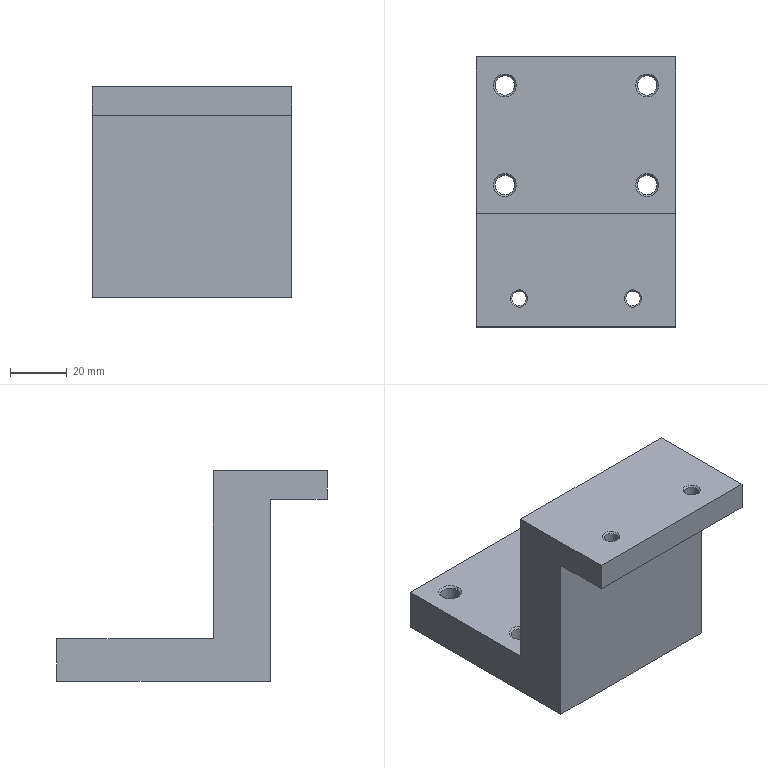Part | SolidWorks | features HoleWzd 2, ICE 2, Extrusion 1 | 1 solid | 34 faces | box 70 x 95 x 74 mm | volume 172756 mm3 | cone 12 | cylinder 12 | plane 10 | commonest cylinder face diameters 6.8 x8 5 x4
STEP:
#1=CARTESIAN_POINT('',(17.5,25.,9.475));
#2=VERTEX_POINT('',#1);
#3=CARTESIAN_POINT('',(22.5,25.,9.475));
#4=VERTEX_POINT('',#3);
#5=CARTESIAN_POINT('',(20.,25.,9.475));
#6=DIRECTION('',(0.,0.,1.));
#7=DIRECTION('',(1.,0.,0.));
#8=AXIS2_PLACEMENT_3D('',#5,#6,#7);
#9=CIRCLE('',#8,2.5);
#10=EDGE_CURVE('',#2,#4,#9,.T.);
#11=ORIENTED_EDGE('',*,*,#10,.F.);
#12=CARTESIAN_POINT('',(16.975,25.,10.));
#13=VERTEX_POINT('',#12);
#14=CARTESIAN_POINT('',(16.975,25.,10.));
#15=DIRECTION('',(-0.7071,0.,0.7071));
#16=VECTOR('',#15,1000.);
#17=LINE('',#14,#16);
#18=EDGE_CURVE('',#2,#13,#17,.T.);
#19=ORIENTED_EDGE('',*,*,#18,.T.);
#20=CARTESIAN_POINT('',(23.025,25.,10.));
#21=VERTEX_POINT('',#20);
#22=CARTESIAN_POINT('',(20.,25.,10.));
#23=DIRECTION('',(0.,0.,1.));
#24=DIRECTION('',(1.,0.,0.));
#25=AXIS2_PLACEMENT_3D('',#22,#23,#24);
#26=CIRCLE('',#25,3.025);
#27=EDGE_CURVE('',#13,#21,#26,.T.);
#28=ORIENTED_EDGE('',*,*,#27,.T.);
#29=CARTESIAN_POINT('',(23.025,25.,10.));
#30=DIRECTION('',(0.7071,0.,0.7071));
#31=VECTOR('',#30,1000.);
#32=LINE('',#29,#31);
#33=EDGE_CURVE('',#4,#21,#32,.T.);
#34=ORIENTED_EDGE('',*,*,#33,.F.);
#35=EDGE_LOOP('',(#11,#19,#28,#34));
#36=FACE_OUTER_BOUND('',#35,.T.);
#37=CARTESIAN_POINT('',(20.,25.,10.));
#38=DIRECTION('',(0.,0.,1.));
#39=DIRECTION('',(1.,0.,0.));
#40=AXIS2_PLACEMENT_3D('',#37,#38,#39);
#41=CONICAL_SURFACE('',#40,3.025,0.7854);
#42=ADVANCED_FACE('',(#36),#41,.F.);
#43=CARTESIAN_POINT('',(17.5,25.,0.));
#44=VERTEX_POINT('',#43);
#45=CARTESIAN_POINT('',(22.5,25.,0.));
#46=VERTEX_POINT('',#45);
#47=CARTESIAN_POINT('',(20.,25.,0.));
#48=DIRECTION('',(0.,0.,1.));
#49=DIRECTION('',(1.,0.,0.));
#50=AXIS2_PLACEMENT_3D('',#47,#48,#49);
#51=CIRCLE('',#50,2.5);
#52=EDGE_CURVE('',#44,#46,#51,.T.);
#53=ORIENTED_EDGE('',*,*,#52,.F.);
#54=CARTESIAN_POINT('',(17.5,25.,10.));
#55=DIRECTION('',(0.,0.,1.));
#56=VECTOR('',#55,1000.);
#57=LINE('',#54,#56);
#58=EDGE_CURVE('',#44,#2,#57,.T.);
#59=ORIENTED_EDGE('',*,*,#58,.T.);
#60=ORIENTED_EDGE('',*,*,#10,.T.);
#61=CARTESIAN_POINT('',(22.5,25.,10.));
#62=DIRECTION('',(0.,0.,1.));
#63=VECTOR('',#62,1000.);
#64=LINE('',#61,#63);
#65=EDGE_CURVE('',#46,#4,#64,.T.);
#66=ORIENTED_EDGE('',*,*,#65,.F.);
#67=EDGE_LOOP('',(#53,#59,#60,#66));
#68=FACE_OUTER_BOUND('',#67,.T.);
#69=CARTESIAN_POINT('',(20.,25.,10.));
#70=DIRECTION('',(0.,0.,1.));
#71=DIRECTION('',(1.,0.,0.));
#72=AXIS2_PLACEMENT_3D('',#69,#70,#71);
#73=CYLINDRICAL_SURFACE('',#72,2.5);
#74=ADVANCED_FACE('',(#68),#73,.F.);
#75=CARTESIAN_POINT('',(-22.5,25.,9.475));
#76=VERTEX_POINT('',#75);
#77=CARTESIAN_POINT('',(-17.5,25.,9.475));
#78=VERTEX_POINT('',#77);
#79=CARTESIAN_POINT('',(-20.,25.,9.475));
#80=DIRECTION('',(0.,0.,1.));
#81=DIRECTION('',(1.,0.,0.));
#82=AXIS2_PLACEMENT_3D('',#79,#80,#81);
#83=CIRCLE('',#82,2.5);
#84=EDGE_CURVE('',#76,#78,#83,.T.);
#85=ORIENTED_EDGE('',*,*,#84,.F.);
#86=CARTESIAN_POINT('',(-23.025,25.,10.));
#87=VERTEX_POINT('',#86);
#88=CARTESIAN_POINT('',(-23.025,25.,10.));
#89=DIRECTION('',(-0.7071,0.,0.7071));
#90=VECTOR('',#89,1000.);
#91=LINE('',#88,#90);
#92=EDGE_CURVE('',#76,#87,#91,.T.);
#93=ORIENTED_EDGE('',*,*,#92,.T.);
#94=CARTESIAN_POINT('',(-16.975,25.,10.));
#95=VERTEX_POINT('',#94);
#96=CARTESIAN_POINT('',(-20.,25.,10.));
#97=DIRECTION('',(0.,0.,1.));
#98=DIRECTION('',(1.,0.,0.));
#99=AXIS2_PLACEMENT_3D('',#96,#97,#98);
#100=CIRCLE('',#99,3.025);
#101=EDGE_CURVE('',#87,#95,#100,.T.);
#102=ORIENTED_EDGE('',*,*,#101,.T.);
#103=CARTESIAN_POINT('',(-16.975,25.,10.));
#104=DIRECTION('',(0.7071,0.,0.7071));
#105=VECTOR('',#104,1000.);
#106=LINE('',#103,#105);
#107=EDGE_CURVE('',#78,#95,#106,.T.);
#108=ORIENTED_EDGE('',*,*,#107,.F.);
#109=EDGE_LOOP('',(#85,#93,#102,#108));
#110=FACE_OUTER_BOUND('',#109,.T.);
#111=CARTESIAN_POINT('',(-20.,25.,10.));
#112=DIRECTION('',(0.,0.,1.));
#113=DIRECTION('',(1.,0.,0.));
#114=AXIS2_PLACEMENT_3D('',#111,#112,#113);
#115=CONICAL_SURFACE('',#114,3.025,0.7854);
#116=ADVANCED_FACE('',(#110),#115,.F.);
#117=CARTESIAN_POINT('',(-22.5,25.,0.));
#118=VERTEX_POINT('',#117);
#119=CARTESIAN_POINT('',(-17.5,25.,0.));
#120=VERTEX_POINT('',#119);
#121=CARTESIAN_POINT('',(-20.,25.,0.));
#122=DIRECTION('',(0.,0.,1.));
#123=DIRECTION('',(1.,0.,0.));
#124=AXIS2_PLACEMENT_3D('',#121,#122,#123);
#125=CIRCLE('',#124,2.5);
#126=EDGE_CURVE('',#118,#120,#125,.T.);
#127=ORIENTED_EDGE('',*,*,#126,.F.);
#128=CARTESIAN_POINT('',(-22.5,25.,10.));
#129=DIRECTION('',(0.,0.,1.));
#130=VECTOR('',#129,1000.);
#131=LINE('',#128,#130);
#132=EDGE_CURVE('',#118,#76,#131,.T.);
#133=ORIENTED_EDGE('',*,*,#132,.T.);
#134=ORIENTED_EDGE('',*,*,#84,.T.);
#135=CARTESIAN_POINT('',(-17.5,25.,10.));
#136=DIRECTION('',(0.,0.,1.));
#137=VECTOR('',#136,1000.);
#138=LINE('',#135,#137);
#139=EDGE_CURVE('',#120,#78,#138,.T.);
#140=ORIENTED_EDGE('',*,*,#139,.F.);
#141=EDGE_LOOP('',(#127,#133,#134,#140));
#142=FACE_OUTER_BOUND('',#141,.T.);
#143=CARTESIAN_POINT('',(-20.,25.,10.));
#144=DIRECTION('',(0.,0.,1.));
#145=DIRECTION('',(1.,0.,0.));
#146=AXIS2_PLACEMENT_3D('',#143,#144,#145);
#147=CYLINDRICAL_SURFACE('',#146,2.5);
#148=ADVANCED_FACE('',(#142),#147,.F.);
#149=CARTESIAN_POINT('',(21.6,100.,-49.625));
#150=VERTEX_POINT('',#149);
#151=CARTESIAN_POINT('',(28.4,100.,-49.625));
#152=VERTEX_POINT('',#151);
#153=CARTESIAN_POINT('',(25.,100.,-49.625));
#154=DIRECTION('',(0.,0.,1.));
#155=DIRECTION('',(1.,0.,0.));
#156=AXIS2_PLACEMENT_3D('',#153,#154,#155);
#157=CIRCLE('',#156,3.4);
#158=EDGE_CURVE('',#150,#152,#157,.T.);
#159=ORIENTED_EDGE('',*,*,#158,.F.);
#160=CARTESIAN_POINT('',(20.975,100.,-49.));
#161=VERTEX_POINT('',#160);
#162=CARTESIAN_POINT('',(20.975,100.,-49.));
#163=DIRECTION('',(-0.7071,0.,0.7071));
#164=VECTOR('',#163,1000.);
#165=LINE('',#162,#164);
#166=EDGE_CURVE('',#150,#161,#165,.T.);
#167=ORIENTED_EDGE('',*,*,#166,.T.);
#168=CARTESIAN_POINT('',(29.025,100.,-49.));
#169=VERTEX_POINT('',#168);
#170=CARTESIAN_POINT('',(25.,100.,-49.));
#171=DIRECTION('',(0.,0.,1.));
#172=DIRECTION('',(1.,0.,0.));
#173=AXIS2_PLACEMENT_3D('',#170,#171,#172);
#174=CIRCLE('',#173,4.025);
#175=EDGE_CURVE('',#161,#169,#174,.T.);
#176=ORIENTED_EDGE('',*,*,#175,.T.);
#177=CARTESIAN_POINT('',(29.025,100.,-49.));
#178=DIRECTION('',(0.7071,0.,0.7071));
#179=VECTOR('',#178,1000.);
#180=LINE('',#177,#179);
#181=EDGE_CURVE('',#152,#169,#180,.T.);
#182=ORIENTED_EDGE('',*,*,#181,.F.);
#183=EDGE_LOOP('',(#159,#167,#176,#182));
#184=FACE_OUTER_BOUND('',#183,.T.);
#185=CARTESIAN_POINT('',(25.,100.,-49.));
#186=DIRECTION('',(0.,0.,1.));
#187=DIRECTION('',(1.,0.,0.));
#188=AXIS2_PLACEMENT_3D('',#185,#186,#187);
#189=CONICAL_SURFACE('',#188,4.025,0.7854);
#190=ADVANCED_FACE('',(#184),#189,.F.);
#191=CARTESIAN_POINT('',(21.6,100.,-64.));
#192=VERTEX_POINT('',#191);
#193=CARTESIAN_POINT('',(28.4,100.,-64.));
#194=VERTEX_POINT('',#193);
#195=CARTESIAN_POINT('',(25.,100.,-64.));
#196=DIRECTION('',(0.,0.,1.));
#197=DIRECTION('',(1.,0.,0.));
#198=AXIS2_PLACEMENT_3D('',#195,#196,#197);
#199=CIRCLE('',#198,3.4);
#200=EDGE_CURVE('',#192,#194,#199,.T.);
#201=ORIENTED_EDGE('',*,*,#200,.F.);
#202=CARTESIAN_POINT('',(21.6,100.,-49.));
#203=DIRECTION('',(0.,0.,1.));
#204=VECTOR('',#203,1000.);
#205=LINE('',#202,#204);
#206=EDGE_CURVE('',#192,#150,#205,.T.);
#207=ORIENTED_EDGE('',*,*,#206,.T.);
#208=ORIENTED_EDGE('',*,*,#158,.T.);
#209=CARTESIAN_POINT('',(28.4,100.,-49.));
#210=DIRECTION('',(0.,0.,1.));
#211=VECTOR('',#210,1000.);
#212=LINE('',#209,#211);
#213=EDGE_CURVE('',#194,#152,#212,.T.);
#214=ORIENTED_EDGE('',*,*,#213,.F.);
#215=EDGE_LOOP('',(#201,#207,#208,#214));
#216=FACE_OUTER_BOUND('',#215,.T.);
#217=CARTESIAN_POINT('',(25.,100.,-49.));
#218=DIRECTION('',(0.,0.,1.));
#219=DIRECTION('',(1.,0.,0.));
#220=AXIS2_PLACEMENT_3D('',#217,#218,#219);
#221=CYLINDRICAL_SURFACE('',#220,3.4);
#222=ADVANCED_FACE('',(#216),#221,.F.);
#223=CARTESIAN_POINT('',(21.6,65.,-49.625));
#224=VERTEX_POINT('',#223);
#225=CARTESIAN_POINT('',(28.4,65.,-49.625));
#226=VERTEX_POINT('',#225);
#227=CARTESIAN_POINT('',(25.,65.,-49.625));
#228=DIRECTION('',(0.,0.,1.));
#229=DIRECTION('',(1.,0.,0.));
#230=AXIS2_PLACEMENT_3D('',#227,#228,#229);
#231=CIRCLE('',#230,3.4);
#232=EDGE_CURVE('',#224,#226,#231,.T.);
#233=ORIENTED_EDGE('',*,*,#232,.F.);
#234=CARTESIAN_POINT('',(20.975,65.,-49.));
#235=VERTEX_POINT('',#234);
#236=CARTESIAN_POINT('',(20.975,65.,-49.));
#237=DIRECTION('',(-0.7071,0.,0.7071));
#238=VECTOR('',#237,1000.);
#239=LINE('',#236,#238);
#240=EDGE_CURVE('',#224,#235,#239,.T.);
#241=ORIENTED_EDGE('',*,*,#240,.T.);
#242=CARTESIAN_POINT('',(29.025,65.,-49.));
#243=VERTEX_POINT('',#242);
#244=CARTESIAN_POINT('',(25.,65.,-49.));
#245=DIRECTION('',(0.,0.,1.));
#246=DIRECTION('',(1.,0.,0.));
#247=AXIS2_PLACEMENT_3D('',#244,#245,#246);
#248=CIRCLE('',#247,4.025);
#249=EDGE_CURVE('',#235,#243,#248,.T.);
#250=ORIENTED_EDGE('',*,*,#249,.T.);
#251=CARTESIAN_POINT('',(29.025,65.,-49.));
#252=DIRECTION('',(0.7071,0.,0.7071));
#253=VECTOR('',#252,1000.);
#254=LINE('',#251,#253);
#255=EDGE_CURVE('',#226,#243,#254,.T.);
#256=ORIENTED_EDGE('',*,*,#255,.F.);
#257=EDGE_LOOP('',(#233,#241,#250,#256));
#258=FACE_OUTER_BOUND('',#257,.T.);
#259=CARTESIAN_POINT('',(25.,65.,-49.));
#260=DIRECTION('',(0.,0.,1.));
#261=DIRECTION('',(1.,0.,0.));
#262=AXIS2_PLACEMENT_3D('',#259,#260,#261);
#263=CONICAL_SURFACE('',#262,4.025,0.7854);
#264=ADVANCED_FACE('',(#258),#263,.F.);
#265=CARTESIAN_POINT('',(21.6,65.,-64.));
#266=VERTEX_POINT('',#265);
#267=CARTESIAN_POINT('',(28.4,65.,-64.));
#268=VERTEX_POINT('',#267);
#269=CARTESIAN_POINT('',(25.,65.,-64.));
#270=DIRECTION('',(0.,0.,1.));
#271=DIRECTION('',(1.,0.,0.));
#272=AXIS2_PLACEMENT_3D('',#269,#270,#271);
#273=CIRCLE('',#272,3.4);
#274=EDGE_CURVE('',#266,#268,#273,.T.);
#275=ORIENTED_EDGE('',*,*,#274,.F.);
#276=CARTESIAN_POINT('',(21.6,65.,-49.));
#277=DIRECTION('',(0.,0.,1.));
#278=VECTOR('',#277,1000.);
#279=LINE('',#276,#278);
#280=EDGE_CURVE('',#266,#224,#279,.T.);
#281=ORIENTED_EDGE('',*,*,#280,.T.);
#282=ORIENTED_EDGE('',*,*,#232,.T.);
#283=CARTESIAN_POINT('',(28.4,65.,-49.));
#284=DIRECTION('',(0.,0.,1.));
#285=VECTOR('',#284,1000.);
#286=LINE('',#283,#285);
#287=EDGE_CURVE('',#268,#226,#286,.T.);
#288=ORIENTED_EDGE('',*,*,#287,.F.);
#289=EDGE_LOOP('',(#275,#281,#282,#288));
#290=FACE_OUTER_BOUND('',#289,.T.);
#291=CARTESIAN_POINT('',(25.,65.,-49.));
#292=DIRECTION('',(0.,0.,1.));
#293=DIRECTION('',(1.,0.,0.));
#294=AXIS2_PLACEMENT_3D('',#291,#292,#293);
#295=CYLINDRICAL_SURFACE('',#294,3.4);
#296=ADVANCED_FACE('',(#290),#295,.F.);
#297=CARTESIAN_POINT('',(-28.4,65.,-49.625));
#298=VERTEX_POINT('',#297);
#299=CARTESIAN_POINT('',(-21.6,65.,-49.625));
#300=VERTEX_POINT('',#299);
#301=CARTESIAN_POINT('',(-25.,65.,-49.625));
#302=DIRECTION('',(0.,0.,1.));
#303=DIRECTION('',(1.,0.,0.));
#304=AXIS2_PLACEMENT_3D('',#301,#302,#303);
#305=CIRCLE('',#304,3.4);
#306=EDGE_CURVE('',#298,#300,#305,.T.);
#307=ORIENTED_EDGE('',*,*,#306,.F.);
#308=CARTESIAN_POINT('',(-29.025,65.,-49.));
#309=VERTEX_POINT('',#308);
#310=CARTESIAN_POINT('',(-29.025,65.,-49.));
#311=DIRECTION('',(-0.7071,0.,0.7071));
#312=VECTOR('',#311,1000.);
#313=LINE('',#310,#312);
#314=EDGE_CURVE('',#298,#309,#313,.T.);
#315=ORIENTED_EDGE('',*,*,#314,.T.);
#316=CARTESIAN_POINT('',(-20.975,65.,-49.));
#317=VERTEX_POINT('',#316);
#318=CARTESIAN_POINT('',(-25.,65.,-49.));
#319=DIRECTION('',(0.,0.,1.));
#320=DIRECTION('',(1.,0.,0.));
#321=AXIS2_PLACEMENT_3D('',#318,#319,#320);
#322=CIRCLE('',#321,4.025);
#323=EDGE_CURVE('',#309,#317,#322,.T.);
#324=ORIENTED_EDGE('',*,*,#323,.T.);
#325=CARTESIAN_POINT('',(-20.975,65.,-49.));
#326=DIRECTION('',(0.7071,0.,0.7071));
#327=VECTOR('',#326,1000.);
#328=LINE('',#325,#327);
#329=EDGE_CURVE('',#300,#317,#328,.T.);
#330=ORIENTED_EDGE('',*,*,#329,.F.);
#331=EDGE_LOOP('',(#307,#315,#324,#330));
#332=FACE_OUTER_BOUND('',#331,.T.);
#333=CARTESIAN_POINT('',(-25.,65.,-49.));
#334=DIRECTION('',(0.,0.,1.));
#335=DIRECTION('',(1.,0.,0.));
#336=AXIS2_PLACEMENT_3D('',#333,#334,#335);
#337=CONICAL_SURFACE('',#336,4.025,0.7854);
#338=ADVANCED_FACE('',(#332),#337,.F.);
#339=CARTESIAN_POINT('',(-28.4,65.,-64.));
#340=VERTEX_POINT('',#339);
#341=CARTESIAN_POINT('',(-21.6,65.,-64.));
#342=VERTEX_POINT('',#341);
#343=CARTESIAN_POINT('',(-25.,65.,-64.));
#344=DIRECTION('',(0.,0.,1.));
#345=DIRECTION('',(1.,0.,0.));
#346=AXIS2_PLACEMENT_3D('',#343,#344,#345);
#347=CIRCLE('',#346,3.4);
#348=EDGE_CURVE('',#340,#342,#347,.T.);
#349=ORIENTED_EDGE('',*,*,#348,.F.);
#350=CARTESIAN_POINT('',(-28.4,65.,-49.));
#351=DIRECTION('',(0.,0.,1.));
#352=VECTOR('',#351,1000.);
#353=LINE('',#350,#352);
#354=EDGE_CURVE('',#340,#298,#353,.T.);
#355=ORIENTED_EDGE('',*,*,#354,.T.);
#356=ORIENTED_EDGE('',*,*,#306,.T.);
#357=CARTESIAN_POINT('',(-21.6,65.,-49.));
#358=DIRECTION('',(0.,0.,1.));
#359=VECTOR('',#358,1000.);
#360=LINE('',#357,#359);
#361=EDGE_CURVE('',#342,#300,#360,.T.);
#362=ORIENTED_EDGE('',*,*,#361,.F.);
#363=EDGE_LOOP('',(#349,#355,#356,#362));
#364=FACE_OUTER_BOUND('',#363,.T.);
#365=CARTESIAN_POINT('',(-25.,65.,-49.));
#366=DIRECTION('',(0.,0.,1.));
#367=DIRECTION('',(1.,0.,0.));
#368=AXIS2_PLACEMENT_3D('',#365,#366,#367);
#369=CYLINDRICAL_SURFACE('',#368,3.4);
#370=ADVANCED_FACE('',(#364),#369,.F.);
#371=CARTESIAN_POINT('',(-28.4,100.,-49.625));
#372=VERTEX_POINT('',#371);
#373=CARTESIAN_POINT('',(-21.6,100.,-49.625));
#374=VERTEX_POINT('',#373);
#375=CARTESIAN_POINT('',(-25.,100.,-49.625));
#376=DIRECTION('',(0.,0.,1.));
#377=DIRECTION('',(1.,0.,0.));
#378=AXIS2_PLACEMENT_3D('',#375,#376,#377);
#379=CIRCLE('',#378,3.4);
#380=EDGE_CURVE('',#372,#374,#379,.T.);
#381=ORIENTED_EDGE('',*,*,#380,.F.);
#382=CARTESIAN_POINT('',(-29.025,100.,-49.));
#383=VERTEX_POINT('',#382);
#384=CARTESIAN_POINT('',(-29.025,100.,-49.));
#385=DIRECTION('',(-0.7071,0.,0.7071));
#386=VECTOR('',#385,1000.);
#387=LINE('',#384,#386);
#388=EDGE_CURVE('',#372,#383,#387,.T.);
#389=ORIENTED_EDGE('',*,*,#388,.T.);
#390=CARTESIAN_POINT('',(-20.975,100.,-49.));
#391=VERTEX_POINT('',#390);
#392=CARTESIAN_POINT('',(-25.,100.,-49.));
#393=DIRECTION('',(0.,0.,1.));
#394=DIRECTION('',(1.,0.,0.));
#395=AXIS2_PLACEMENT_3D('',#392,#393,#394);
#396=CIRCLE('',#395,4.025);
#397=EDGE_CURVE('',#383,#391,#396,.T.);
#398=ORIENTED_EDGE('',*,*,#397,.T.);
#399=CARTESIAN_POINT('',(-20.975,100.,-49.));
#400=DIRECTION('',(0.7071,0.,0.7071));
#401=VECTOR('',#400,1000.);
#402=LINE('',#399,#401);
#403=EDGE_CURVE('',#374,#391,#402,.T.);
#404=ORIENTED_EDGE('',*,*,#403,.F.);
#405=EDGE_LOOP('',(#381,#389,#398,#404));
#406=FACE_OUTER_BOUND('',#405,.T.);
#407=CARTESIAN_POINT('',(-25.,100.,-49.));
#408=DIRECTION('',(0.,0.,1.));
#409=DIRECTION('',(1.,0.,0.));
#410=AXIS2_PLACEMENT_3D('',#407,#408,#409);
#411=CONICAL_SURFACE('',#410,4.025,0.7854);
#412=ADVANCED_FACE('',(#406),#411,.F.);
#413=CARTESIAN_POINT('',(-28.4,100.,-64.));
#414=VERTEX_POINT('',#413);
#415=CARTESIAN_POINT('',(-21.6,100.,-64.));
#416=VERTEX_POINT('',#415);
#417=CARTESIAN_POINT('',(-25.,100.,-64.));
#418=DIRECTION('',(0.,0.,1.));
#419=DIRECTION('',(1.,0.,0.));
#420=AXIS2_PLACEMENT_3D('',#417,#418,#419);
#421=CIRCLE('',#420,3.4);
#422=EDGE_CURVE('',#414,#416,#421,.T.);
#423=ORIENTED_EDGE('',*,*,#422,.F.);
#424=CARTESIAN_POINT('',(-28.4,100.,-49.));
#425=DIRECTION('',(0.,0.,1.));
#426=VECTOR('',#425,1000.);
#427=LINE('',#424,#426);
#428=EDGE_CURVE('',#414,#372,#427,.T.);
#429=ORIENTED_EDGE('',*,*,#428,.T.);
#430=ORIENTED_EDGE('',*,*,#380,.T.);
#431=CARTESIAN_POINT('',(-21.6,100.,-49.));
#432=DIRECTION('',(0.,0.,1.));
#433=VECTOR('',#432,1000.);
#434=LINE('',#431,#433);
#435=EDGE_CURVE('',#416,#374,#434,.T.);
#436=ORIENTED_EDGE('',*,*,#435,.F.);
#437=EDGE_LOOP('',(#423,#429,#430,#436));
#438=FACE_OUTER_BOUND('',#437,.T.);
#439=CARTESIAN_POINT('',(-25.,100.,-49.));
#440=DIRECTION('',(0.,0.,1.));
#441=DIRECTION('',(1.,0.,0.));
#442=AXIS2_PLACEMENT_3D('',#439,#440,#441);
#443=CYLINDRICAL_SURFACE('',#442,3.4);
#444=ADVANCED_FACE('',(#438),#443,.F.);
#445=CARTESIAN_POINT('',(25.,100.,-49.));
#446=DIRECTION('',(0.,0.,1.));
#447=DIRECTION('',(1.,0.,0.));
#448=AXIS2_PLACEMENT_3D('',#445,#446,#447);
#449=CIRCLE('',#448,4.025);
#450=EDGE_CURVE('',#169,#161,#449,.T.);
#451=ORIENTED_EDGE('',*,*,#450,.F.);
#452=ORIENTED_EDGE('',*,*,#175,.F.);
#453=EDGE_LOOP('',(#451,#452));
#454=FACE_BOUND('',#453,.T.);
#455=CARTESIAN_POINT('',(25.,65.,-49.));
#456=DIRECTION('',(0.,0.,1.));
#457=DIRECTION('',(1.,0.,0.));
#458=AXIS2_PLACEMENT_3D('',#455,#456,#457);
#459=CIRCLE('',#458,4.025);
#460=EDGE_CURVE('',#243,#235,#459,.T.);
#461=ORIENTED_EDGE('',*,*,#460,.F.);
#462=ORIENTED_EDGE('',*,*,#249,.F.);
#463=EDGE_LOOP('',(#461,#462));
#464=FACE_BOUND('',#463,.T.);
#465=CARTESIAN_POINT('',(-25.,100.,-49.));
#466=DIRECTION('',(0.,0.,1.));
#467=DIRECTION('',(1.,0.,0.));
#468=AXIS2_PLACEMENT_3D('',#465,#466,#467);
#469=CIRCLE('',#468,4.025);
#470=EDGE_CURVE('',#391,#383,#469,.T.);
#471=ORIENTED_EDGE('',*,*,#470,.F.);
#472=ORIENTED_EDGE('',*,*,#397,.F.);
#473=EDGE_LOOP('',(#471,#472));
#474=FACE_BOUND('',#473,.T.);
#475=CARTESIAN_POINT('',(-35.,55.,-49.));
#476=VERTEX_POINT('',#475);
#477=CARTESIAN_POINT('',(35.,55.,-49.));
#478=VERTEX_POINT('',#477);
#479=CARTESIAN_POINT('',(35.,55.,-49.));
#480=DIRECTION('',(1.,0.,0.));
#481=VECTOR('',#480,1000.);
#482=LINE('',#479,#481);
#483=EDGE_CURVE('',#476,#478,#482,.T.);
#484=ORIENTED_EDGE('',*,*,#483,.T.);
#485=CARTESIAN_POINT('',(35.,110.,-49.));
#486=VERTEX_POINT('',#485);
#487=CARTESIAN_POINT('',(35.,110.,-49.));
#488=DIRECTION('',(0.,-1.,0.));
#489=VECTOR('',#488,1000.);
#490=LINE('',#487,#489);
#491=EDGE_CURVE('',#486,#478,#490,.T.);
#492=ORIENTED_EDGE('',*,*,#491,.F.);
#493=CARTESIAN_POINT('',(-35.,110.,-49.));
#494=VERTEX_POINT('',#493);
#495=CARTESIAN_POINT('',(35.,110.,-49.));
#496=DIRECTION('',(1.,0.,0.));
#497=VECTOR('',#496,1000.);
#498=LINE('',#495,#497);
#499=EDGE_CURVE('',#494,#486,#498,.T.);
#500=ORIENTED_EDGE('',*,*,#499,.F.);
#501=CARTESIAN_POINT('',(-35.,110.,-49.));
#502=DIRECTION('',(0.,-1.,0.));
#503=VECTOR('',#502,1000.);
#504=LINE('',#501,#503);
#505=EDGE_CURVE('',#494,#476,#504,.T.);
#506=ORIENTED_EDGE('',*,*,#505,.T.);
#507=EDGE_LOOP('',(#484,#492,#500,#506));
#508=FACE_OUTER_BOUND('',#507,.T.);
#509=CARTESIAN_POINT('',(-25.,65.,-49.));
#510=DIRECTION('',(0.,0.,1.));
#511=DIRECTION('',(1.,0.,0.));
#512=AXIS2_PLACEMENT_3D('',#509,#510,#511);
#513=CIRCLE('',#512,4.025);
#514=EDGE_CURVE('',#317,#309,#513,.T.);
#515=ORIENTED_EDGE('',*,*,#514,.F.);
#516=ORIENTED_EDGE('',*,*,#323,.F.);
#517=EDGE_LOOP('',(#515,#516));
#518=FACE_BOUND('',#517,.T.);
#519=CARTESIAN_POINT('',(35.,110.,-49.));
#520=DIRECTION('',(0.,0.,-1.));
#521=DIRECTION('',(-1.,0.,0.));
#522=AXIS2_PLACEMENT_3D('',#519,#520,#521);
#523=PLANE('',#522);
#524=ADVANCED_FACE('',(#454,#464,#474,#508,#518),#523,.F.);
#525=ORIENTED_EDGE('',*,*,#483,.F.);
#526=CARTESIAN_POINT('',(-35.,55.,10.));
#527=VERTEX_POINT('',#526);
#528=CARTESIAN_POINT('',(-35.,55.,10.));
#529=DIRECTION('',(0.,0.,-1.));
#530=VECTOR('',#529,1000.);
#531=LINE('',#528,#530);
#532=EDGE_CURVE('',#527,#476,#531,.T.);
#533=ORIENTED_EDGE('',*,*,#532,.F.);
#534=CARTESIAN_POINT('',(35.,55.,10.));
#535=VERTEX_POINT('',#534);
#536=CARTESIAN_POINT('',(-35.,55.,10.));
#537=DIRECTION('',(-1.,0.,0.));
#538=VECTOR('',#537,1000.);
#539=LINE('',#536,#538);
#540=EDGE_CURVE('',#535,#527,#539,.T.);
#541=ORIENTED_EDGE('',*,*,#540,.F.);
#542=CARTESIAN_POINT('',(35.,55.,10.));
#543=DIRECTION('',(0.,0.,-1.));
#544=VECTOR('',#543,1000.);
#545=LINE('',#542,#544);
#546=EDGE_CURVE('',#535,#478,#545,.T.);
#547=ORIENTED_EDGE('',*,*,#546,.T.);
#548=EDGE_LOOP('',(#525,#533,#541,#547));
#549=FACE_OUTER_BOUND('',#548,.T.);
#550=CARTESIAN_POINT('',(-35.,55.,10.));
#551=DIRECTION('',(0.,-1.,0.));
#552=DIRECTION('',(0.,0.,-1.));
#553=AXIS2_PLACEMENT_3D('',#550,#551,#552);
#554=PLANE('',#553);
#555=ADVANCED_FACE('',(#549),#554,.F.);
#556=CARTESIAN_POINT('',(-35.,35.,0.));
#557=VERTEX_POINT('',#556);
#558=CARTESIAN_POINT('',(35.,35.,0.));
#559=VERTEX_POINT('',#558);
#560=CARTESIAN_POINT('',(-35.,35.,0.));
#561=DIRECTION('',(1.,0.,0.));
#562=VECTOR('',#561,1000.);
#563=LINE('',#560,#562);
#564=EDGE_CURVE('',#557,#559,#563,.T.);
#565=ORIENTED_EDGE('',*,*,#564,.F.);
#566=CARTESIAN_POINT('',(-35.,35.,-64.));
#567=VERTEX_POINT('',#566);
#568=CARTESIAN_POINT('',(-35.,35.,10.));
#569=DIRECTION('',(0.,0.,-1.));
#570=VECTOR('',#569,1000.);
#571=LINE('',#568,#570);
#572=EDGE_CURVE('',#557,#567,#571,.T.);
#573=ORIENTED_EDGE('',*,*,#572,.T.);
#574=CARTESIAN_POINT('',(35.,35.,-64.));
#575=VERTEX_POINT('',#574);
#576=CARTESIAN_POINT('',(-35.,35.,-64.));
#577=DIRECTION('',(1.,0.,0.));
#578=VECTOR('',#577,1000.);
#579=LINE('',#576,#578);
#580=EDGE_CURVE('',#567,#575,#579,.T.);
#581=ORIENTED_EDGE('',*,*,#580,.T.);
#582=CARTESIAN_POINT('',(35.,35.,10.));
#583=DIRECTION('',(0.,0.,-1.));
#584=VECTOR('',#583,1000.);
#585=LINE('',#582,#584);
#586=EDGE_CURVE('',#559,#575,#585,.T.);
#587=ORIENTED_EDGE('',*,*,#586,.F.);
#588=EDGE_LOOP('',(#565,#573,#581,#587));
#589=FACE_OUTER_BOUND('',#588,.T.);
#590=CARTESIAN_POINT('',(-35.,35.,10.));
#591=DIRECTION('',(0.,1.,0.));
#592=DIRECTION('',(0.,0.,1.));
#593=AXIS2_PLACEMENT_3D('',#590,#591,#592);
#594=PLANE('',#593);
#595=ADVANCED_FACE('',(#589),#594,.F.);
#596=CARTESIAN_POINT('',(35.,15.,10.));
#597=VERTEX_POINT('',#596);
#598=CARTESIAN_POINT('',(35.,55.,10.));
#599=DIRECTION('',(0.,1.,0.));
#600=VECTOR('',#599,1000.);
#601=LINE('',#598,#600);
#602=EDGE_CURVE('',#597,#535,#601,.T.);
#603=ORIENTED_EDGE('',*,*,#602,.F.);
#604=CARTESIAN_POINT('',(35.,15.,0.));
#605=VERTEX_POINT('',#604);
#606=CARTESIAN_POINT('',(35.,15.,10.));
#607=DIRECTION('',(0.,0.,1.));
#608=VECTOR('',#607,1000.);
#609=LINE('',#606,#608);
#610=EDGE_CURVE('',#605,#597,#609,.T.);
#611=ORIENTED_EDGE('',*,*,#610,.F.);
#612=CARTESIAN_POINT('',(35.,15.,0.));
#613=DIRECTION('',(0.,1.,0.));
#614=VECTOR('',#613,1000.);
#615=LINE('',#612,#614);
#616=EDGE_CURVE('',#605,#559,#615,.T.);
#617=ORIENTED_EDGE('',*,*,#616,.T.);
#618=ORIENTED_EDGE('',*,*,#586,.T.);
#619=CARTESIAN_POINT('',(35.,110.,-64.));
#620=VERTEX_POINT('',#619);
#621=CARTESIAN_POINT('',(35.,55.,-64.));
#622=DIRECTION('',(0.,1.,0.));
#623=VECTOR('',#622,1000.);
#624=LINE('',#621,#623);
#625=EDGE_CURVE('',#575,#620,#624,.T.);
#626=ORIENTED_EDGE('',*,*,#625,.T.);
#627=CARTESIAN_POINT('',(35.,110.,-64.));
#628=DIRECTION('',(0.,0.,-1.));
#629=VECTOR('',#628,1000.);
#630=LINE('',#627,#629);
#631=EDGE_CURVE('',#486,#620,#630,.T.);
#632=ORIENTED_EDGE('',*,*,#631,.F.);
#633=ORIENTED_EDGE('',*,*,#491,.T.);
#634=ORIENTED_EDGE('',*,*,#546,.F.);
#635=EDGE_LOOP('',(#603,#611,#617,#618,#626,#632,#633,#634));
#636=FACE_OUTER_BOUND('',#635,.T.);
#637=CARTESIAN_POINT('',(35.,55.,10.));
#638=DIRECTION('',(-1.,0.,0.));
#639=DIRECTION('',(0.,0.,1.));
#640=AXIS2_PLACEMENT_3D('',#637,#638,#639);
#641=PLANE('',#640);
#642=ADVANCED_FACE('',(#636),#641,.F.);
#643=ORIENTED_EDGE('',*,*,#532,.T.);
#644=ORIENTED_EDGE('',*,*,#505,.F.);
#645=CARTESIAN_POINT('',(-35.,110.,-64.));
#646=VERTEX_POINT('',#645);
#647=CARTESIAN_POINT('',(-35.,110.,-64.));
#648=DIRECTION('',(0.,0.,1.));
#649=VECTOR('',#648,1000.);
#650=LINE('',#647,#649);
#651=EDGE_CURVE('',#646,#494,#650,.T.);
#652=ORIENTED_EDGE('',*,*,#651,.F.);
#653=CARTESIAN_POINT('',(-35.,55.,-64.));
#654=DIRECTION('',(0.,-1.,0.));
#655=VECTOR('',#654,1000.);
#656=LINE('',#653,#655);
#657=EDGE_CURVE('',#646,#567,#656,.T.);
#658=ORIENTED_EDGE('',*,*,#657,.T.);
#659=ORIENTED_EDGE('',*,*,#572,.F.);
#660=CARTESIAN_POINT('',(-35.,15.,0.));
#661=VERTEX_POINT('',#660);
#662=CARTESIAN_POINT('',(-35.,15.,0.));
#663=DIRECTION('',(0.,1.,0.));
#664=VECTOR('',#663,1000.);
#665=LINE('',#662,#664);
#666=EDGE_CURVE('',#661,#557,#665,.T.);
#667=ORIENTED_EDGE('',*,*,#666,.F.);
#668=CARTESIAN_POINT('',(-35.,15.,10.));
#669=VERTEX_POINT('',#668);
#670=CARTESIAN_POINT('',(-35.,15.,10.));
#671=DIRECTION('',(0.,0.,-1.));
#672=VECTOR('',#671,1000.);
#673=LINE('',#670,#672);
#674=EDGE_CURVE('',#669,#661,#673,.T.);
#675=ORIENTED_EDGE('',*,*,#674,.F.);
#676=CARTESIAN_POINT('',(-35.,55.,10.));
#677=DIRECTION('',(0.,-1.,0.));
#678=VECTOR('',#677,1000.);
#679=LINE('',#676,#678);
#680=EDGE_CURVE('',#527,#669,#679,.T.);
#681=ORIENTED_EDGE('',*,*,#680,.F.);
#682=EDGE_LOOP('',(#643,#644,#652,#658,#659,#667,#675,#681));
#683=FACE_OUTER_BOUND('',#682,.T.);
#684=CARTESIAN_POINT('',(-35.,55.,10.));
#685=DIRECTION('',(1.,0.,0.));
#686=DIRECTION('',(0.,0.,-1.));
#687=AXIS2_PLACEMENT_3D('',#684,#685,#686);
#688=PLANE('',#687);
#689=ADVANCED_FACE('',(#683),#688,.F.);
#690=CARTESIAN_POINT('',(20.,25.,10.));
#691=DIRECTION('',(0.,0.,1.));
#692=DIRECTION('',(1.,0.,0.));
#693=AXIS2_PLACEMENT_3D('',#690,#691,#692);
#694=CIRCLE('',#693,3.025);
#695=EDGE_CURVE('',#21,#13,#694,.T.);
#696=ORIENTED_EDGE('',*,*,#695,.F.);
#697=ORIENTED_EDGE('',*,*,#27,.F.);
#698=EDGE_LOOP('',(#696,#697));
#699=FACE_BOUND('',#698,.T.);
#700=CARTESIAN_POINT('',(-20.,25.,10.));
#701=DIRECTION('',(0.,0.,1.));
#702=DIRECTION('',(1.,0.,0.));
#703=AXIS2_PLACEMENT_3D('',#700,#701,#702);
#704=CIRCLE('',#703,3.025);
#705=EDGE_CURVE('',#95,#87,#704,.T.);
#706=ORIENTED_EDGE('',*,*,#705,.F.);
#707=ORIENTED_EDGE('',*,*,#101,.F.);
#708=EDGE_LOOP('',(#706,#707));
#709=FACE_BOUND('',#708,.T.);
#710=ORIENTED_EDGE('',*,*,#602,.T.);
#711=ORIENTED_EDGE('',*,*,#540,.T.);
#712=ORIENTED_EDGE('',*,*,#680,.T.);
#713=CARTESIAN_POINT('',(-35.,15.,10.));
#714=DIRECTION('',(-1.,0.,0.));
#715=VECTOR('',#714,1000.);
#716=LINE('',#713,#715);
#717=EDGE_CURVE('',#597,#669,#716,.T.);
#718=ORIENTED_EDGE('',*,*,#717,.F.);
#719=EDGE_LOOP('',(#710,#711,#712,#718));
#720=FACE_OUTER_BOUND('',#719,.T.);
#721=CARTESIAN_POINT('',(0.,0.,10.));
#722=DIRECTION('',(0.,0.,1.));
#723=DIRECTION('',(1.,0.,0.));
#724=AXIS2_PLACEMENT_3D('',#721,#722,#723);
#725=PLANE('',#724);
#726=ADVANCED_FACE('',(#699,#709,#720),#725,.T.);
#727=CARTESIAN_POINT('',(25.,100.,-64.));
#728=DIRECTION('',(0.,0.,1.));
#729=DIRECTION('',(1.,0.,0.));
#730=AXIS2_PLACEMENT_3D('',#727,#728,#729);
#731=CIRCLE('',#730,3.4);
#732=EDGE_CURVE('',#194,#192,#731,.T.);
#733=ORIENTED_EDGE('',*,*,#732,.T.);
#734=ORIENTED_EDGE('',*,*,#200,.T.);
#735=EDGE_LOOP('',(#733,#734));
#736=FACE_BOUND('',#735,.T.);
#737=CARTESIAN_POINT('',(25.,65.,-64.));
#738=DIRECTION('',(0.,0.,1.));
#739=DIRECTION('',(1.,0.,0.));
#740=AXIS2_PLACEMENT_3D('',#737,#738,#739);
#741=CIRCLE('',#740,3.4);
#742=EDGE_CURVE('',#268,#266,#741,.T.);
#743=ORIENTED_EDGE('',*,*,#742,.T.);
#744=ORIENTED_EDGE('',*,*,#274,.T.);
#745=EDGE_LOOP('',(#743,#744));
#746=FACE_BOUND('',#745,.T.);
#747=CARTESIAN_POINT('',(-25.,65.,-64.));
#748=DIRECTION('',(0.,0.,1.));
#749=DIRECTION('',(1.,0.,0.));
#750=AXIS2_PLACEMENT_3D('',#747,#748,#749);
#751=CIRCLE('',#750,3.4);
#752=EDGE_CURVE('',#342,#340,#751,.T.);
#753=ORIENTED_EDGE('',*,*,#752,.T.);
#754=ORIENTED_EDGE('',*,*,#348,.T.);
#755=EDGE_LOOP('',(#753,#754));
#756=FACE_BOUND('',#755,.T.);
#757=CARTESIAN_POINT('',(-25.,100.,-64.));
#758=DIRECTION('',(0.,0.,1.));
#759=DIRECTION('',(1.,0.,0.));
#760=AXIS2_PLACEMENT_3D('',#757,#758,#759);
#761=CIRCLE('',#760,3.4);
#762=EDGE_CURVE('',#416,#414,#761,.T.);
#763=ORIENTED_EDGE('',*,*,#762,.T.);
#764=ORIENTED_EDGE('',*,*,#422,.T.);
#765=EDGE_LOOP('',(#763,#764));
#766=FACE_BOUND('',#765,.T.);
#767=ORIENTED_EDGE('',*,*,#625,.F.);
#768=ORIENTED_EDGE('',*,*,#580,.F.);
#769=ORIENTED_EDGE('',*,*,#657,.F.);
#770=CARTESIAN_POINT('',(35.,110.,-64.));
#771=DIRECTION('',(-1.,0.,0.));
#772=VECTOR('',#771,1000.);
#773=LINE('',#770,#772);
#774=EDGE_CURVE('',#620,#646,#773,.T.);
#775=ORIENTED_EDGE('',*,*,#774,.F.);
#776=EDGE_LOOP('',(#767,#768,#769,#775));
#777=FACE_OUTER_BOUND('',#776,.T.);
#778=CARTESIAN_POINT('',(0.,0.,-64.));
#779=DIRECTION('',(0.,0.,1.));
#780=DIRECTION('',(1.,0.,0.));
#781=AXIS2_PLACEMENT_3D('',#778,#779,#780);
#782=PLANE('',#781);
#783=ADVANCED_FACE('',(#736,#746,#756,#766,#777),#782,.F.);
#784=CARTESIAN_POINT('',(20.,25.,0.));
#785=DIRECTION('',(0.,0.,1.));
#786=DIRECTION('',(1.,0.,0.));
#787=AXIS2_PLACEMENT_3D('',#784,#785,#786);
#788=CIRCLE('',#787,2.5);
#789=EDGE_CURVE('',#46,#44,#788,.T.);
#790=ORIENTED_EDGE('',*,*,#789,.T.);
#791=ORIENTED_EDGE('',*,*,#52,.T.);
#792=EDGE_LOOP('',(#790,#791));
#793=FACE_BOUND('',#792,.T.);
#794=CARTESIAN_POINT('',(-20.,25.,0.));
#795=DIRECTION('',(0.,0.,1.));
#796=DIRECTION('',(1.,0.,0.));
#797=AXIS2_PLACEMENT_3D('',#794,#795,#796);
#798=CIRCLE('',#797,2.5);
#799=EDGE_CURVE('',#120,#118,#798,.T.);
#800=ORIENTED_EDGE('',*,*,#799,.T.);
#801=ORIENTED_EDGE('',*,*,#126,.T.);
#802=EDGE_LOOP('',(#800,#801));
#803=FACE_BOUND('',#802,.T.);
#804=ORIENTED_EDGE('',*,*,#564,.T.);
#805=ORIENTED_EDGE('',*,*,#616,.F.);
#806=CARTESIAN_POINT('',(-35.,15.,0.));
#807=DIRECTION('',(1.,0.,0.));
#808=VECTOR('',#807,1000.);
#809=LINE('',#806,#808);
#810=EDGE_CURVE('',#661,#605,#809,.T.);
#811=ORIENTED_EDGE('',*,*,#810,.F.);
#812=ORIENTED_EDGE('',*,*,#666,.T.);
#813=EDGE_LOOP('',(#804,#805,#811,#812));
#814=FACE_OUTER_BOUND('',#813,.T.);
#815=CARTESIAN_POINT('',(-35.,15.,0.));
#816=DIRECTION('',(0.,0.,1.));
#817=DIRECTION('',(1.,0.,0.));
#818=AXIS2_PLACEMENT_3D('',#815,#816,#817);
#819=PLANE('',#818);
#820=ADVANCED_FACE('',(#793,#803,#814),#819,.F.);
#821=ORIENTED_EDGE('',*,*,#674,.T.);
#822=ORIENTED_EDGE('',*,*,#810,.T.);
#823=ORIENTED_EDGE('',*,*,#610,.T.);
#824=ORIENTED_EDGE('',*,*,#717,.T.);
#825=EDGE_LOOP('',(#821,#822,#823,#824));
#826=FACE_OUTER_BOUND('',#825,.T.);
#827=CARTESIAN_POINT('',(0.,15.,0.));
#828=DIRECTION('',(0.,-1.,0.));
#829=DIRECTION('',(0.,0.,-1.));
#830=AXIS2_PLACEMENT_3D('',#827,#828,#829);
#831=PLANE('',#830);
#832=ADVANCED_FACE('',(#826),#831,.T.);
#833=ORIENTED_EDGE('',*,*,#631,.T.);
#834=ORIENTED_EDGE('',*,*,#774,.T.);
#835=ORIENTED_EDGE('',*,*,#651,.T.);
#836=ORIENTED_EDGE('',*,*,#499,.T.);
#837=EDGE_LOOP('',(#833,#834,#835,#836));
#838=FACE_OUTER_BOUND('',#837,.T.);
#839=CARTESIAN_POINT('',(0.,110.,0.));
#840=DIRECTION('',(0.,-1.,0.));
#841=DIRECTION('',(0.,0.,-1.));
#842=AXIS2_PLACEMENT_3D('',#839,#840,#841);
#843=PLANE('',#842);
#844=ADVANCED_FACE('',(#838),#843,.F.);
#845=ORIENTED_EDGE('',*,*,#428,.F.);
#846=ORIENTED_EDGE('',*,*,#762,.F.);
#847=ORIENTED_EDGE('',*,*,#435,.T.);
#848=CARTESIAN_POINT('',(-25.,100.,-49.625));
#849=DIRECTION('',(0.,0.,1.));
#850=DIRECTION('',(1.,0.,0.));
#851=AXIS2_PLACEMENT_3D('',#848,#849,#850);
#852=CIRCLE('',#851,3.4);
#853=EDGE_CURVE('',#374,#372,#852,.T.);
#854=ORIENTED_EDGE('',*,*,#853,.T.);
#855=EDGE_LOOP('',(#845,#846,#847,#854));
#856=FACE_OUTER_BOUND('',#855,.T.);
#857=CARTESIAN_POINT('',(-25.,100.,-49.));
#858=DIRECTION('',(0.,0.,1.));
#859=DIRECTION('',(1.,0.,0.));
#860=AXIS2_PLACEMENT_3D('',#857,#858,#859);
#861=CYLINDRICAL_SURFACE('',#860,3.4);
#862=ADVANCED_FACE('',(#856),#861,.F.);
#863=ORIENTED_EDGE('',*,*,#388,.F.);
#864=ORIENTED_EDGE('',*,*,#853,.F.);
#865=ORIENTED_EDGE('',*,*,#403,.T.);
#866=ORIENTED_EDGE('',*,*,#470,.T.);
#867=EDGE_LOOP('',(#863,#864,#865,#866));
#868=FACE_OUTER_BOUND('',#867,.T.);
#869=CARTESIAN_POINT('',(-25.,100.,-49.));
#870=DIRECTION('',(0.,0.,1.));
#871=DIRECTION('',(1.,0.,0.));
#872=AXIS2_PLACEMENT_3D('',#869,#870,#871);
#873=CONICAL_SURFACE('',#872,4.025,0.7854);
#874=ADVANCED_FACE('',(#868),#873,.F.);
#875=ORIENTED_EDGE('',*,*,#354,.F.);
#876=ORIENTED_EDGE('',*,*,#752,.F.);
#877=ORIENTED_EDGE('',*,*,#361,.T.);
#878=CARTESIAN_POINT('',(-25.,65.,-49.625));
#879=DIRECTION('',(0.,0.,1.));
#880=DIRECTION('',(1.,0.,0.));
#881=AXIS2_PLACEMENT_3D('',#878,#879,#880);
#882=CIRCLE('',#881,3.4);
#883=EDGE_CURVE('',#300,#298,#882,.T.);
#884=ORIENTED_EDGE('',*,*,#883,.T.);
#885=EDGE_LOOP('',(#875,#876,#877,#884));
#886=FACE_OUTER_BOUND('',#885,.T.);
#887=CARTESIAN_POINT('',(-25.,65.,-49.));
#888=DIRECTION('',(0.,0.,1.));
#889=DIRECTION('',(1.,0.,0.));
#890=AXIS2_PLACEMENT_3D('',#887,#888,#889);
#891=CYLINDRICAL_SURFACE('',#890,3.4);
#892=ADVANCED_FACE('',(#886),#891,.F.);
#893=ORIENTED_EDGE('',*,*,#314,.F.);
#894=ORIENTED_EDGE('',*,*,#883,.F.);
#895=ORIENTED_EDGE('',*,*,#329,.T.);
#896=ORIENTED_EDGE('',*,*,#514,.T.);
#897=EDGE_LOOP('',(#893,#894,#895,#896));
#898=FACE_OUTER_BOUND('',#897,.T.);
#899=CARTESIAN_POINT('',(-25.,65.,-49.));
#900=DIRECTION('',(0.,0.,1.));
#901=DIRECTION('',(1.,0.,0.));
#902=AXIS2_PLACEMENT_3D('',#899,#900,#901);
#903=CONICAL_SURFACE('',#902,4.025,0.7854);
#904=ADVANCED_FACE('',(#898),#903,.F.);
#905=ORIENTED_EDGE('',*,*,#280,.F.);
#906=ORIENTED_EDGE('',*,*,#742,.F.);
#907=ORIENTED_EDGE('',*,*,#287,.T.);
#908=CARTESIAN_POINT('',(25.,65.,-49.625));
#909=DIRECTION('',(0.,0.,1.));
#910=DIRECTION('',(1.,0.,0.));
#911=AXIS2_PLACEMENT_3D('',#908,#909,#910);
#912=CIRCLE('',#911,3.4);
#913=EDGE_CURVE('',#226,#224,#912,.T.);
#914=ORIENTED_EDGE('',*,*,#913,.T.);
#915=EDGE_LOOP('',(#905,#906,#907,#914));
#916=FACE_OUTER_BOUND('',#915,.T.);
#917=CARTESIAN_POINT('',(25.,65.,-49.));
#918=DIRECTION('',(0.,0.,1.));
#919=DIRECTION('',(1.,0.,0.));
#920=AXIS2_PLACEMENT_3D('',#917,#918,#919);
#921=CYLINDRICAL_SURFACE('',#920,3.4);
#922=ADVANCED_FACE('',(#916),#921,.F.);
#923=ORIENTED_EDGE('',*,*,#240,.F.);
#924=ORIENTED_EDGE('',*,*,#913,.F.);
#925=ORIENTED_EDGE('',*,*,#255,.T.);
#926=ORIENTED_EDGE('',*,*,#460,.T.);
#927=EDGE_LOOP('',(#923,#924,#925,#926));
#928=FACE_OUTER_BOUND('',#927,.T.);
#929=CARTESIAN_POINT('',(25.,65.,-49.));
#930=DIRECTION('',(0.,0.,1.));
#931=DIRECTION('',(1.,0.,0.));
#932=AXIS2_PLACEMENT_3D('',#929,#930,#931);
#933=CONICAL_SURFACE('',#932,4.025,0.7854);
#934=ADVANCED_FACE('',(#928),#933,.F.);
#935=ORIENTED_EDGE('',*,*,#206,.F.);
#936=ORIENTED_EDGE('',*,*,#732,.F.);
#937=ORIENTED_EDGE('',*,*,#213,.T.);
#938=CARTESIAN_POINT('',(25.,100.,-49.625));
#939=DIRECTION('',(0.,0.,1.));
#940=DIRECTION('',(1.,0.,0.));
#941=AXIS2_PLACEMENT_3D('',#938,#939,#940);
#942=CIRCLE('',#941,3.4);
#943=EDGE_CURVE('',#152,#150,#942,.T.);
#944=ORIENTED_EDGE('',*,*,#943,.T.);
#945=EDGE_LOOP('',(#935,#936,#937,#944));
#946=FACE_OUTER_BOUND('',#945,.T.);
#947=CARTESIAN_POINT('',(25.,100.,-49.));
#948=DIRECTION('',(0.,0.,1.));
#949=DIRECTION('',(1.,0.,0.));
#950=AXIS2_PLACEMENT_3D('',#947,#948,#949);
#951=CYLINDRICAL_SURFACE('',#950,3.4);
#952=ADVANCED_FACE('',(#946),#951,.F.);
#953=ORIENTED_EDGE('',*,*,#166,.F.);
#954=ORIENTED_EDGE('',*,*,#943,.F.);
#955=ORIENTED_EDGE('',*,*,#181,.T.);
#956=ORIENTED_EDGE('',*,*,#450,.T.);
#957=EDGE_LOOP('',(#953,#954,#955,#956));
#958=FACE_OUTER_BOUND('',#957,.T.);
#959=CARTESIAN_POINT('',(25.,100.,-49.));
#960=DIRECTION('',(0.,0.,1.));
#961=DIRECTION('',(1.,0.,0.));
#962=AXIS2_PLACEMENT_3D('',#959,#960,#961);
#963=CONICAL_SURFACE('',#962,4.025,0.7854);
#964=ADVANCED_FACE('',(#958),#963,.F.);
#965=ORIENTED_EDGE('',*,*,#132,.F.);
#966=ORIENTED_EDGE('',*,*,#799,.F.);
#967=ORIENTED_EDGE('',*,*,#139,.T.);
#968=CARTESIAN_POINT('',(-20.,25.,9.475));
#969=DIRECTION('',(0.,0.,1.));
#970=DIRECTION('',(1.,0.,0.));
#971=AXIS2_PLACEMENT_3D('',#968,#969,#970);
#972=CIRCLE('',#971,2.5);
#973=EDGE_CURVE('',#78,#76,#972,.T.);
#974=ORIENTED_EDGE('',*,*,#973,.T.);
#975=EDGE_LOOP('',(#965,#966,#967,#974));
#976=FACE_OUTER_BOUND('',#975,.T.);
#977=CARTESIAN_POINT('',(-20.,25.,10.));
#978=DIRECTION('',(0.,0.,1.));
#979=DIRECTION('',(1.,0.,0.));
#980=AXIS2_PLACEMENT_3D('',#977,#978,#979);
#981=CYLINDRICAL_SURFACE('',#980,2.5);
#982=ADVANCED_FACE('',(#976),#981,.F.);
#983=ORIENTED_EDGE('',*,*,#92,.F.);
#984=ORIENTED_EDGE('',*,*,#973,.F.);
#985=ORIENTED_EDGE('',*,*,#107,.T.);
#986=ORIENTED_EDGE('',*,*,#705,.T.);
#987=EDGE_LOOP('',(#983,#984,#985,#986));
#988=FACE_OUTER_BOUND('',#987,.T.);
#989=CARTESIAN_POINT('',(-20.,25.,10.));
#990=DIRECTION('',(0.,0.,1.));
#991=DIRECTION('',(1.,0.,0.));
#992=AXIS2_PLACEMENT_3D('',#989,#990,#991);
#993=CONICAL_SURFACE('',#992,3.025,0.7854);
#994=ADVANCED_FACE('',(#988),#993,.F.);
#995=ORIENTED_EDGE('',*,*,#58,.F.);
#996=ORIENTED_EDGE('',*,*,#789,.F.);
#997=ORIENTED_EDGE('',*,*,#65,.T.);
#998=CARTESIAN_POINT('',(20.,25.,9.475));
#999=DIRECTION('',(0.,0.,1.));
#1000=DIRECTION('',(1.,0.,0.));
#1001=AXIS2_PLACEMENT_3D('',#998,#999,#1000);
#1002=CIRCLE('',#1001,2.5);
#1003=EDGE_CURVE('',#4,#2,#1002,.T.);
#1004=ORIENTED_EDGE('',*,*,#1003,.T.);
#1005=EDGE_LOOP('',(#995,#996,#997,#1004));
#1006=FACE_OUTER_BOUND('',#1005,.T.);
#1007=CARTESIAN_POINT('',(20.,25.,10.));
#1008=DIRECTION('',(0.,0.,1.));
#1009=DIRECTION('',(1.,0.,0.));
#1010=AXIS2_PLACEMENT_3D('',#1007,#1008,#1009);
#1011=CYLINDRICAL_SURFACE('',#1010,2.5);
#1012=ADVANCED_FACE('',(#1006),#1011,.F.);
#1013=ORIENTED_EDGE('',*,*,#18,.F.);
#1014=ORIENTED_EDGE('',*,*,#1003,.F.);
#1015=ORIENTED_EDGE('',*,*,#33,.T.);
#1016=ORIENTED_EDGE('',*,*,#695,.T.);
#1017=EDGE_LOOP('',(#1013,#1014,#1015,#1016));
#1018=FACE_OUTER_BOUND('',#1017,.T.);
#1019=CARTESIAN_POINT('',(20.,25.,10.));
#1020=DIRECTION('',(0.,0.,1.));
#1021=DIRECTION('',(1.,0.,0.));
#1022=AXIS2_PLACEMENT_3D('',#1019,#1020,#1021);
#1023=CONICAL_SURFACE('',#1022,3.025,0.7854);
#1024=ADVANCED_FACE('',(#1018),#1023,.F.);
#1025=CLOSED_SHELL('',(#42,#74,#116,#148,#190,#222,#264,#296,#338,#370,#412,#444,#524,#555,#595,#642,#689,#726,#783,#820,#832,#844,#862,#874,#892,#904,#922,#934,#952,#964,#982,#994,#1012,#1024));
#1026=MANIFOLD_SOLID_BREP('',#1025);
#1027=CARTESIAN_POINT('',(0.,0.,0.));
#1028=DIRECTION('',(0.,0.,1.));
#1029=DIRECTION('',(1.,0.,0.));
#1030=AXIS2_PLACEMENT_3D('',#1027,#1028,#1029);
#1031=(LENGTH_UNIT()NAMED_UNIT(*)SI_UNIT(.MILLI.,.METRE.));
#1032=UNCERTAINTY_MEASURE_WITH_UNIT(LENGTH_MEASURE(0.00001),#1031,'','');
#1033=(NAMED_UNIT(*)PLANE_ANGLE_UNIT()SI_UNIT($,.RADIAN.));
#1034=(NAMED_UNIT(*)SI_UNIT($,.STERADIAN.)SOLID_ANGLE_UNIT());
#1035=(GEOMETRIC_REPRESENTATION_CONTEXT(3)GLOBAL_UNCERTAINTY_ASSIGNED_CONTEXT((#1032))GLOBAL_UNIT_ASSIGNED_CONTEXT((#1031,#1033,#1034))REPRESENTATION_CONTEXT('',''));
#1036=ADVANCED_BREP_SHAPE_REPRESENTATION('',(#1026,#1030),#1035);